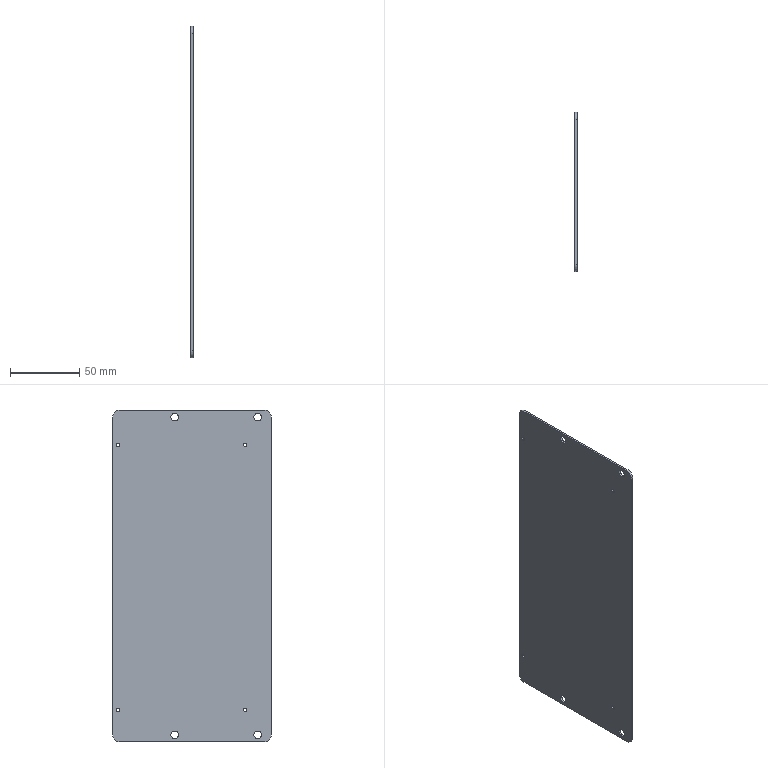Part | NX | features BREP 1 | 1 solid | 18 faces | box 1.5 x 115 x 240 mm | volume 41196 mm3 | cylinder 12 | plane 6 | commonest cylinder face diameters 2.5 x4 5.5 x4 10 x4
STEP:
#1=CARTESIAN_POINT('',(0.,-47.5,117.75));
#2=VERTEX_POINT('',#1);
#3=CARTESIAN_POINT('',(0.,-47.5,115.));
#4=DIRECTION('',(-1.,0.,0.));
#5=DIRECTION('',(0.,0.,1.));
#6=AXIS2_PLACEMENT_3D('',#3,#4,#5);
#7=CIRCLE('',#6,2.75);
#8=EDGE_CURVE('',#2,#2,#7,.T.);
#9=ORIENTED_EDGE('',*,*,#8,.T.);
#10=EDGE_LOOP('',(#9));
#11=FACE_BOUND('',#10,.T.);
#12=CARTESIAN_POINT('',(1.5,-47.5,117.75));
#13=VERTEX_POINT('',#12);
#14=CARTESIAN_POINT('',(1.5,-47.5,115.));
#15=DIRECTION('',(-1.,0.,0.));
#16=DIRECTION('',(0.,0.,1.));
#17=AXIS2_PLACEMENT_3D('',#14,#15,#16);
#18=CIRCLE('',#17,2.75);
#19=EDGE_CURVE('',#13,#13,#18,.T.);
#20=ORIENTED_EDGE('',*,*,#19,.F.);
#21=EDGE_LOOP('',(#20));
#22=FACE_BOUND('',#21,.T.);
#23=CARTESIAN_POINT('',(0.,-47.5,115.));
#24=DIRECTION('',(-1.,0.,0.));
#25=DIRECTION('',(0.,0.,1.));
#26=AXIS2_PLACEMENT_3D('',#23,#24,#25);
#27=CYLINDRICAL_SURFACE('',#26,2.75);
#28=ADVANCED_FACE('',(#11,#22),#27,.F.);
#29=CARTESIAN_POINT('',(0.,12.5,-112.25));
#30=VERTEX_POINT('',#29);
#31=CARTESIAN_POINT('',(0.,12.5,-115.));
#32=DIRECTION('',(-1.,0.,0.));
#33=DIRECTION('',(0.,0.,1.));
#34=AXIS2_PLACEMENT_3D('',#31,#32,#33);
#35=CIRCLE('',#34,2.75);
#36=EDGE_CURVE('',#30,#30,#35,.T.);
#37=ORIENTED_EDGE('',*,*,#36,.T.);
#38=EDGE_LOOP('',(#37));
#39=FACE_BOUND('',#38,.T.);
#40=CARTESIAN_POINT('',(1.5,12.5,-112.25));
#41=VERTEX_POINT('',#40);
#42=CARTESIAN_POINT('',(1.5,12.5,-115.));
#43=DIRECTION('',(-1.,0.,0.));
#44=DIRECTION('',(0.,0.,1.));
#45=AXIS2_PLACEMENT_3D('',#42,#43,#44);
#46=CIRCLE('',#45,2.75);
#47=EDGE_CURVE('',#41,#41,#46,.T.);
#48=ORIENTED_EDGE('',*,*,#47,.F.);
#49=EDGE_LOOP('',(#48));
#50=FACE_BOUND('',#49,.T.);
#51=CARTESIAN_POINT('',(0.,12.5,-115.));
#52=DIRECTION('',(-1.,0.,0.));
#53=DIRECTION('',(0.,0.,1.));
#54=AXIS2_PLACEMENT_3D('',#51,#52,#53);
#55=CYLINDRICAL_SURFACE('',#54,2.75);
#56=ADVANCED_FACE('',(#39,#50),#55,.F.);
#57=CARTESIAN_POINT('',(0.,-47.5,-112.25));
#58=VERTEX_POINT('',#57);
#59=CARTESIAN_POINT('',(0.,-47.5,-115.));
#60=DIRECTION('',(-1.,0.,0.));
#61=DIRECTION('',(0.,0.,1.));
#62=AXIS2_PLACEMENT_3D('',#59,#60,#61);
#63=CIRCLE('',#62,2.75);
#64=EDGE_CURVE('',#58,#58,#63,.T.);
#65=ORIENTED_EDGE('',*,*,#64,.T.);
#66=EDGE_LOOP('',(#65));
#67=FACE_BOUND('',#66,.T.);
#68=CARTESIAN_POINT('',(1.5,-47.5,-112.25));
#69=VERTEX_POINT('',#68);
#70=CARTESIAN_POINT('',(1.5,-47.5,-115.));
#71=DIRECTION('',(-1.,0.,0.));
#72=DIRECTION('',(0.,0.,1.));
#73=AXIS2_PLACEMENT_3D('',#70,#71,#72);
#74=CIRCLE('',#73,2.75);
#75=EDGE_CURVE('',#69,#69,#74,.T.);
#76=ORIENTED_EDGE('',*,*,#75,.F.);
#77=EDGE_LOOP('',(#76));
#78=FACE_BOUND('',#77,.T.);
#79=CARTESIAN_POINT('',(0.,-47.5,-115.));
#80=DIRECTION('',(-1.,0.,0.));
#81=DIRECTION('',(0.,0.,1.));
#82=AXIS2_PLACEMENT_3D('',#79,#80,#81);
#83=CYLINDRICAL_SURFACE('',#82,2.75);
#84=ADVANCED_FACE('',(#67,#78),#83,.F.);
#85=CARTESIAN_POINT('',(0.,12.5,117.75));
#86=VERTEX_POINT('',#85);
#87=CARTESIAN_POINT('',(0.,12.5,115.));
#88=DIRECTION('',(-1.,0.,0.));
#89=DIRECTION('',(0.,0.,1.));
#90=AXIS2_PLACEMENT_3D('',#87,#88,#89);
#91=CIRCLE('',#90,2.75);
#92=EDGE_CURVE('',#86,#86,#91,.T.);
#93=ORIENTED_EDGE('',*,*,#92,.T.);
#94=EDGE_LOOP('',(#93));
#95=FACE_BOUND('',#94,.T.);
#96=CARTESIAN_POINT('',(1.5,12.5,117.75));
#97=VERTEX_POINT('',#96);
#98=CARTESIAN_POINT('',(1.5,12.5,115.));
#99=DIRECTION('',(-1.,0.,0.));
#100=DIRECTION('',(0.,0.,1.));
#101=AXIS2_PLACEMENT_3D('',#98,#99,#100);
#102=CIRCLE('',#101,2.75);
#103=EDGE_CURVE('',#97,#97,#102,.T.);
#104=ORIENTED_EDGE('',*,*,#103,.F.);
#105=EDGE_LOOP('',(#104));
#106=FACE_BOUND('',#105,.T.);
#107=CARTESIAN_POINT('',(0.,12.5,115.));
#108=DIRECTION('',(-1.,0.,0.));
#109=DIRECTION('',(0.,0.,1.));
#110=AXIS2_PLACEMENT_3D('',#107,#108,#109);
#111=CYLINDRICAL_SURFACE('',#110,2.75);
#112=ADVANCED_FACE('',(#95,#106),#111,.F.);
#113=CARTESIAN_POINT('',(0.,53.5,96.25));
#114=VERTEX_POINT('',#113);
#115=CARTESIAN_POINT('',(0.,53.5,95.));
#116=DIRECTION('',(-1.,0.,0.));
#117=DIRECTION('',(0.,0.,1.));
#118=AXIS2_PLACEMENT_3D('',#115,#116,#117);
#119=CIRCLE('',#118,1.25);
#120=EDGE_CURVE('',#114,#114,#119,.T.);
#121=ORIENTED_EDGE('',*,*,#120,.T.);
#122=EDGE_LOOP('',(#121));
#123=FACE_BOUND('',#122,.T.);
#124=CARTESIAN_POINT('',(1.5,53.5,96.25));
#125=VERTEX_POINT('',#124);
#126=CARTESIAN_POINT('',(1.5,53.5,95.));
#127=DIRECTION('',(-1.,0.,0.));
#128=DIRECTION('',(0.,0.,1.));
#129=AXIS2_PLACEMENT_3D('',#126,#127,#128);
#130=CIRCLE('',#129,1.25);
#131=EDGE_CURVE('',#125,#125,#130,.T.);
#132=ORIENTED_EDGE('',*,*,#131,.F.);
#133=EDGE_LOOP('',(#132));
#134=FACE_BOUND('',#133,.T.);
#135=CARTESIAN_POINT('',(0.,53.5,95.));
#136=DIRECTION('',(-1.,0.,0.));
#137=DIRECTION('',(0.,0.,1.));
#138=AXIS2_PLACEMENT_3D('',#135,#136,#137);
#139=CYLINDRICAL_SURFACE('',#138,1.25);
#140=ADVANCED_FACE('',(#123,#134),#139,.F.);
#141=CARTESIAN_POINT('',(0.,53.5,-95.75));
#142=VERTEX_POINT('',#141);
#143=CARTESIAN_POINT('',(0.,53.5,-97.));
#144=DIRECTION('',(-1.,0.,0.));
#145=DIRECTION('',(0.,0.,1.));
#146=AXIS2_PLACEMENT_3D('',#143,#144,#145);
#147=CIRCLE('',#146,1.25);
#148=EDGE_CURVE('',#142,#142,#147,.T.);
#149=ORIENTED_EDGE('',*,*,#148,.T.);
#150=EDGE_LOOP('',(#149));
#151=FACE_BOUND('',#150,.T.);
#152=CARTESIAN_POINT('',(1.5,53.5,-95.75));
#153=VERTEX_POINT('',#152);
#154=CARTESIAN_POINT('',(1.5,53.5,-97.));
#155=DIRECTION('',(-1.,0.,0.));
#156=DIRECTION('',(0.,0.,1.));
#157=AXIS2_PLACEMENT_3D('',#154,#155,#156);
#158=CIRCLE('',#157,1.25);
#159=EDGE_CURVE('',#153,#153,#158,.T.);
#160=ORIENTED_EDGE('',*,*,#159,.F.);
#161=EDGE_LOOP('',(#160));
#162=FACE_BOUND('',#161,.T.);
#163=CARTESIAN_POINT('',(0.,53.5,-97.));
#164=DIRECTION('',(-1.,0.,0.));
#165=DIRECTION('',(0.,0.,1.));
#166=AXIS2_PLACEMENT_3D('',#163,#164,#165);
#167=CYLINDRICAL_SURFACE('',#166,1.25);
#168=ADVANCED_FACE('',(#151,#162),#167,.F.);
#169=CARTESIAN_POINT('',(0.,-38.5,-95.75));
#170=VERTEX_POINT('',#169);
#171=CARTESIAN_POINT('',(0.,-38.5,-97.));
#172=DIRECTION('',(-1.,0.,0.));
#173=DIRECTION('',(0.,0.,1.));
#174=AXIS2_PLACEMENT_3D('',#171,#172,#173);
#175=CIRCLE('',#174,1.25);
#176=EDGE_CURVE('',#170,#170,#175,.T.);
#177=ORIENTED_EDGE('',*,*,#176,.T.);
#178=EDGE_LOOP('',(#177));
#179=FACE_BOUND('',#178,.T.);
#180=CARTESIAN_POINT('',(1.5,-38.5,-95.75));
#181=VERTEX_POINT('',#180);
#182=CARTESIAN_POINT('',(1.5,-38.5,-97.));
#183=DIRECTION('',(-1.,0.,0.));
#184=DIRECTION('',(0.,0.,1.));
#185=AXIS2_PLACEMENT_3D('',#182,#183,#184);
#186=CIRCLE('',#185,1.25);
#187=EDGE_CURVE('',#181,#181,#186,.T.);
#188=ORIENTED_EDGE('',*,*,#187,.F.);
#189=EDGE_LOOP('',(#188));
#190=FACE_BOUND('',#189,.T.);
#191=CARTESIAN_POINT('',(0.,-38.5,-97.));
#192=DIRECTION('',(-1.,0.,0.));
#193=DIRECTION('',(0.,0.,1.));
#194=AXIS2_PLACEMENT_3D('',#191,#192,#193);
#195=CYLINDRICAL_SURFACE('',#194,1.25);
#196=ADVANCED_FACE('',(#179,#190),#195,.F.);
#197=CARTESIAN_POINT('',(0.,-38.5,96.25));
#198=VERTEX_POINT('',#197);
#199=CARTESIAN_POINT('',(0.,-38.5,95.));
#200=DIRECTION('',(-1.,0.,0.));
#201=DIRECTION('',(0.,0.,1.));
#202=AXIS2_PLACEMENT_3D('',#199,#200,#201);
#203=CIRCLE('',#202,1.25);
#204=EDGE_CURVE('',#198,#198,#203,.T.);
#205=ORIENTED_EDGE('',*,*,#204,.T.);
#206=EDGE_LOOP('',(#205));
#207=FACE_BOUND('',#206,.T.);
#208=CARTESIAN_POINT('',(1.5,-38.5,96.25));
#209=VERTEX_POINT('',#208);
#210=CARTESIAN_POINT('',(1.5,-38.5,95.));
#211=DIRECTION('',(-1.,0.,0.));
#212=DIRECTION('',(0.,0.,1.));
#213=AXIS2_PLACEMENT_3D('',#210,#211,#212);
#214=CIRCLE('',#213,1.25);
#215=EDGE_CURVE('',#209,#209,#214,.T.);
#216=ORIENTED_EDGE('',*,*,#215,.F.);
#217=EDGE_LOOP('',(#216));
#218=FACE_BOUND('',#217,.T.);
#219=CARTESIAN_POINT('',(0.,-38.5,95.));
#220=DIRECTION('',(-1.,0.,0.));
#221=DIRECTION('',(0.,0.,1.));
#222=AXIS2_PLACEMENT_3D('',#219,#220,#221);
#223=CYLINDRICAL_SURFACE('',#222,1.25);
#224=ADVANCED_FACE('',(#207,#218),#223,.F.);
#225=ORIENTED_EDGE('',*,*,#19,.T.);
#226=EDGE_LOOP('',(#225));
#227=FACE_BOUND('',#226,.T.);
#228=ORIENTED_EDGE('',*,*,#47,.T.);
#229=EDGE_LOOP('',(#228));
#230=FACE_BOUND('',#229,.T.);
#231=ORIENTED_EDGE('',*,*,#75,.T.);
#232=EDGE_LOOP('',(#231));
#233=FACE_BOUND('',#232,.T.);
#234=ORIENTED_EDGE('',*,*,#103,.T.);
#235=EDGE_LOOP('',(#234));
#236=FACE_BOUND('',#235,.T.);
#237=CARTESIAN_POINT('',(1.5,-52.5,-120.));
#238=VERTEX_POINT('',#237);
#239=CARTESIAN_POINT('',(1.5,52.5,-120.));
#240=VERTEX_POINT('',#239);
#241=CARTESIAN_POINT('',(1.5,57.5,-120.));
#242=DIRECTION('',(0.,1.,0.));
#243=VECTOR('',#242,1000.);
#244=LINE('',#241,#243);
#245=EDGE_CURVE('',#238,#240,#244,.T.);
#246=ORIENTED_EDGE('',*,*,#245,.T.);
#247=CARTESIAN_POINT('',(1.5,57.5,-115.));
#248=VERTEX_POINT('',#247);
#249=CARTESIAN_POINT('',(1.5,52.5,-115.));
#250=DIRECTION('',(1.,0.,0.));
#251=DIRECTION('',(0.,0.,-1.));
#252=AXIS2_PLACEMENT_3D('',#249,#250,#251);
#253=CIRCLE('',#252,5.);
#254=EDGE_CURVE('',#240,#248,#253,.T.);
#255=ORIENTED_EDGE('',*,*,#254,.T.);
#256=CARTESIAN_POINT('',(1.5,57.5,115.));
#257=VERTEX_POINT('',#256);
#258=CARTESIAN_POINT('',(1.5,57.5,120.));
#259=DIRECTION('',(0.,0.,1.));
#260=VECTOR('',#259,1000.);
#261=LINE('',#258,#260);
#262=EDGE_CURVE('',#248,#257,#261,.T.);
#263=ORIENTED_EDGE('',*,*,#262,.T.);
#264=CARTESIAN_POINT('',(1.5,52.5,120.));
#265=VERTEX_POINT('',#264);
#266=CARTESIAN_POINT('',(1.5,52.5,115.));
#267=DIRECTION('',(1.,0.,0.));
#268=DIRECTION('',(0.,0.,-1.));
#269=AXIS2_PLACEMENT_3D('',#266,#267,#268);
#270=CIRCLE('',#269,5.);
#271=EDGE_CURVE('',#257,#265,#270,.T.);
#272=ORIENTED_EDGE('',*,*,#271,.T.);
#273=CARTESIAN_POINT('',(1.5,-52.5,120.));
#274=VERTEX_POINT('',#273);
#275=CARTESIAN_POINT('',(1.5,57.5,120.));
#276=DIRECTION('',(0.,-1.,0.));
#277=VECTOR('',#276,1000.);
#278=LINE('',#275,#277);
#279=EDGE_CURVE('',#265,#274,#278,.T.);
#280=ORIENTED_EDGE('',*,*,#279,.T.);
#281=CARTESIAN_POINT('',(1.5,-57.5,115.));
#282=VERTEX_POINT('',#281);
#283=CARTESIAN_POINT('',(1.5,-52.5,115.));
#284=DIRECTION('',(1.,0.,0.));
#285=DIRECTION('',(0.,0.,-1.));
#286=AXIS2_PLACEMENT_3D('',#283,#284,#285);
#287=CIRCLE('',#286,5.);
#288=EDGE_CURVE('',#274,#282,#287,.T.);
#289=ORIENTED_EDGE('',*,*,#288,.T.);
#290=CARTESIAN_POINT('',(1.5,-57.5,-115.));
#291=VERTEX_POINT('',#290);
#292=CARTESIAN_POINT('',(1.5,-57.5,120.));
#293=DIRECTION('',(0.,0.,-1.));
#294=VECTOR('',#293,1000.);
#295=LINE('',#292,#294);
#296=EDGE_CURVE('',#282,#291,#295,.T.);
#297=ORIENTED_EDGE('',*,*,#296,.T.);
#298=CARTESIAN_POINT('',(1.5,-52.5,-115.));
#299=DIRECTION('',(1.,0.,0.));
#300=DIRECTION('',(0.,0.,-1.));
#301=AXIS2_PLACEMENT_3D('',#298,#299,#300);
#302=CIRCLE('',#301,5.);
#303=EDGE_CURVE('',#291,#238,#302,.T.);
#304=ORIENTED_EDGE('',*,*,#303,.T.);
#305=EDGE_LOOP('',(#246,#255,#263,#272,#280,#289,#297,#304));
#306=FACE_BOUND('',#305,.T.);
#307=ORIENTED_EDGE('',*,*,#215,.T.);
#308=EDGE_LOOP('',(#307));
#309=FACE_BOUND('',#308,.T.);
#310=ORIENTED_EDGE('',*,*,#187,.T.);
#311=EDGE_LOOP('',(#310));
#312=FACE_BOUND('',#311,.T.);
#313=ORIENTED_EDGE('',*,*,#159,.T.);
#314=EDGE_LOOP('',(#313));
#315=FACE_BOUND('',#314,.T.);
#316=ORIENTED_EDGE('',*,*,#131,.T.);
#317=EDGE_LOOP('',(#316));
#318=FACE_BOUND('',#317,.T.);
#319=CARTESIAN_POINT('',(1.5,0.,0.));
#320=DIRECTION('',(1.,0.,0.));
#321=DIRECTION('',(0.,0.,-1.));
#322=AXIS2_PLACEMENT_3D('',#319,#320,#321);
#323=PLANE('',#322);
#324=ADVANCED_FACE('',(#227,#230,#233,#236,#306,#309,#312,#315,#318),#323,.T.);
#325=CARTESIAN_POINT('',(0.,-52.5,-120.));
#326=VERTEX_POINT('',#325);
#327=CARTESIAN_POINT('',(0.,52.5,-120.));
#328=VERTEX_POINT('',#327);
#329=CARTESIAN_POINT('',(0.,57.5,-120.));
#330=DIRECTION('',(0.,1.,0.));
#331=VECTOR('',#330,1000.);
#332=LINE('',#329,#331);
#333=EDGE_CURVE('',#326,#328,#332,.T.);
#334=ORIENTED_EDGE('',*,*,#333,.T.);
#335=CARTESIAN_POINT('',(1.5,52.5,-120.));
#336=DIRECTION('',(1.,0.,0.));
#337=VECTOR('',#336,1000.);
#338=LINE('',#335,#337);
#339=EDGE_CURVE('',#328,#240,#338,.T.);
#340=ORIENTED_EDGE('',*,*,#339,.T.);
#341=ORIENTED_EDGE('',*,*,#245,.F.);
#342=CARTESIAN_POINT('',(1.5,-52.5,-120.));
#343=DIRECTION('',(-1.,0.,0.));
#344=VECTOR('',#343,1000.);
#345=LINE('',#342,#344);
#346=EDGE_CURVE('',#238,#326,#345,.T.);
#347=ORIENTED_EDGE('',*,*,#346,.T.);
#348=EDGE_LOOP('',(#334,#340,#341,#347));
#349=FACE_BOUND('',#348,.T.);
#350=CARTESIAN_POINT('',(1.5,57.5,-120.));
#351=DIRECTION('',(0.,0.,1.));
#352=DIRECTION('',(1.,0.,0.));
#353=AXIS2_PLACEMENT_3D('',#350,#351,#352);
#354=PLANE('',#353);
#355=ADVANCED_FACE('',(#349),#354,.F.);
#356=ORIENTED_EDGE('',*,*,#262,.F.);
#357=CARTESIAN_POINT('',(0.,57.5,-115.));
#358=VERTEX_POINT('',#357);
#359=CARTESIAN_POINT('',(1.5,57.5,-115.));
#360=DIRECTION('',(-1.,0.,0.));
#361=VECTOR('',#360,1000.);
#362=LINE('',#359,#361);
#363=EDGE_CURVE('',#248,#358,#362,.T.);
#364=ORIENTED_EDGE('',*,*,#363,.T.);
#365=CARTESIAN_POINT('',(0.,57.5,115.));
#366=VERTEX_POINT('',#365);
#367=CARTESIAN_POINT('',(0.,57.5,120.));
#368=DIRECTION('',(0.,0.,1.));
#369=VECTOR('',#368,1000.);
#370=LINE('',#367,#369);
#371=EDGE_CURVE('',#358,#366,#370,.T.);
#372=ORIENTED_EDGE('',*,*,#371,.T.);
#373=CARTESIAN_POINT('',(1.5,57.5,115.));
#374=DIRECTION('',(1.,0.,0.));
#375=VECTOR('',#374,1000.);
#376=LINE('',#373,#375);
#377=EDGE_CURVE('',#366,#257,#376,.T.);
#378=ORIENTED_EDGE('',*,*,#377,.T.);
#379=EDGE_LOOP('',(#356,#364,#372,#378));
#380=FACE_BOUND('',#379,.T.);
#381=CARTESIAN_POINT('',(1.5,57.5,120.));
#382=DIRECTION('',(0.,-1.,0.));
#383=DIRECTION('',(0.,0.,-1.));
#384=AXIS2_PLACEMENT_3D('',#381,#382,#383);
#385=PLANE('',#384);
#386=ADVANCED_FACE('',(#380),#385,.F.);
#387=CARTESIAN_POINT('',(0.,52.5,120.));
#388=VERTEX_POINT('',#387);
#389=CARTESIAN_POINT('',(0.,-52.5,120.));
#390=VERTEX_POINT('',#389);
#391=CARTESIAN_POINT('',(0.,57.5,120.));
#392=DIRECTION('',(0.,-1.,0.));
#393=VECTOR('',#392,1000.);
#394=LINE('',#391,#393);
#395=EDGE_CURVE('',#388,#390,#394,.T.);
#396=ORIENTED_EDGE('',*,*,#395,.T.);
#397=CARTESIAN_POINT('',(1.5,-52.5,120.));
#398=DIRECTION('',(1.,0.,0.));
#399=VECTOR('',#398,1000.);
#400=LINE('',#397,#399);
#401=EDGE_CURVE('',#390,#274,#400,.T.);
#402=ORIENTED_EDGE('',*,*,#401,.T.);
#403=ORIENTED_EDGE('',*,*,#279,.F.);
#404=CARTESIAN_POINT('',(1.5,52.5,120.));
#405=DIRECTION('',(-1.,0.,0.));
#406=VECTOR('',#405,1000.);
#407=LINE('',#404,#406);
#408=EDGE_CURVE('',#265,#388,#407,.T.);
#409=ORIENTED_EDGE('',*,*,#408,.T.);
#410=EDGE_LOOP('',(#396,#402,#403,#409));
#411=FACE_BOUND('',#410,.T.);
#412=CARTESIAN_POINT('',(1.5,57.5,120.));
#413=DIRECTION('',(0.,0.,-1.));
#414=DIRECTION('',(-1.,0.,0.));
#415=AXIS2_PLACEMENT_3D('',#412,#413,#414);
#416=PLANE('',#415);
#417=ADVANCED_FACE('',(#411),#416,.F.);
#418=CARTESIAN_POINT('',(0.,-57.5,115.));
#419=VERTEX_POINT('',#418);
#420=CARTESIAN_POINT('',(0.,-57.5,-115.));
#421=VERTEX_POINT('',#420);
#422=CARTESIAN_POINT('',(0.,-57.5,120.));
#423=DIRECTION('',(0.,0.,-1.));
#424=VECTOR('',#423,1000.);
#425=LINE('',#422,#424);
#426=EDGE_CURVE('',#419,#421,#425,.T.);
#427=ORIENTED_EDGE('',*,*,#426,.T.);
#428=CARTESIAN_POINT('',(1.5,-57.5,-115.));
#429=DIRECTION('',(1.,0.,0.));
#430=VECTOR('',#429,1000.);
#431=LINE('',#428,#430);
#432=EDGE_CURVE('',#421,#291,#431,.T.);
#433=ORIENTED_EDGE('',*,*,#432,.T.);
#434=ORIENTED_EDGE('',*,*,#296,.F.);
#435=CARTESIAN_POINT('',(1.5,-57.5,115.));
#436=DIRECTION('',(-1.,0.,0.));
#437=VECTOR('',#436,1000.);
#438=LINE('',#435,#437);
#439=EDGE_CURVE('',#282,#419,#438,.T.);
#440=ORIENTED_EDGE('',*,*,#439,.T.);
#441=EDGE_LOOP('',(#427,#433,#434,#440));
#442=FACE_BOUND('',#441,.T.);
#443=CARTESIAN_POINT('',(1.5,-57.5,120.));
#444=DIRECTION('',(0.,1.,0.));
#445=DIRECTION('',(0.,0.,1.));
#446=AXIS2_PLACEMENT_3D('',#443,#444,#445);
#447=PLANE('',#446);
#448=ADVANCED_FACE('',(#442),#447,.F.);
#449=ORIENTED_EDGE('',*,*,#8,.F.);
#450=EDGE_LOOP('',(#449));
#451=FACE_BOUND('',#450,.T.);
#452=ORIENTED_EDGE('',*,*,#36,.F.);
#453=EDGE_LOOP('',(#452));
#454=FACE_BOUND('',#453,.T.);
#455=ORIENTED_EDGE('',*,*,#64,.F.);
#456=EDGE_LOOP('',(#455));
#457=FACE_BOUND('',#456,.T.);
#458=ORIENTED_EDGE('',*,*,#92,.F.);
#459=EDGE_LOOP('',(#458));
#460=FACE_BOUND('',#459,.T.);
#461=ORIENTED_EDGE('',*,*,#120,.F.);
#462=EDGE_LOOP('',(#461));
#463=FACE_BOUND('',#462,.T.);
#464=ORIENTED_EDGE('',*,*,#148,.F.);
#465=EDGE_LOOP('',(#464));
#466=FACE_BOUND('',#465,.T.);
#467=ORIENTED_EDGE('',*,*,#176,.F.);
#468=EDGE_LOOP('',(#467));
#469=FACE_BOUND('',#468,.T.);
#470=ORIENTED_EDGE('',*,*,#204,.F.);
#471=EDGE_LOOP('',(#470));
#472=FACE_BOUND('',#471,.T.);
#473=ORIENTED_EDGE('',*,*,#371,.F.);
#474=CARTESIAN_POINT('',(0.,52.5,-115.));
#475=DIRECTION('',(-1.,0.,0.));
#476=DIRECTION('',(0.,0.,-1.));
#477=AXIS2_PLACEMENT_3D('',#474,#475,#476);
#478=CIRCLE('',#477,5.);
#479=EDGE_CURVE('',#358,#328,#478,.T.);
#480=ORIENTED_EDGE('',*,*,#479,.T.);
#481=ORIENTED_EDGE('',*,*,#333,.F.);
#482=CARTESIAN_POINT('',(0.,-52.5,-115.));
#483=DIRECTION('',(-1.,0.,0.));
#484=DIRECTION('',(0.,0.,-1.));
#485=AXIS2_PLACEMENT_3D('',#482,#483,#484);
#486=CIRCLE('',#485,5.);
#487=EDGE_CURVE('',#326,#421,#486,.T.);
#488=ORIENTED_EDGE('',*,*,#487,.T.);
#489=ORIENTED_EDGE('',*,*,#426,.F.);
#490=CARTESIAN_POINT('',(0.,-52.5,115.));
#491=DIRECTION('',(-1.,0.,0.));
#492=DIRECTION('',(0.,0.,-1.));
#493=AXIS2_PLACEMENT_3D('',#490,#491,#492);
#494=CIRCLE('',#493,5.);
#495=EDGE_CURVE('',#419,#390,#494,.T.);
#496=ORIENTED_EDGE('',*,*,#495,.T.);
#497=ORIENTED_EDGE('',*,*,#395,.F.);
#498=CARTESIAN_POINT('',(0.,52.5,115.));
#499=DIRECTION('',(-1.,0.,0.));
#500=DIRECTION('',(0.,0.,-1.));
#501=AXIS2_PLACEMENT_3D('',#498,#499,#500);
#502=CIRCLE('',#501,5.);
#503=EDGE_CURVE('',#388,#366,#502,.T.);
#504=ORIENTED_EDGE('',*,*,#503,.T.);
#505=EDGE_LOOP('',(#473,#480,#481,#488,#489,#496,#497,#504));
#506=FACE_BOUND('',#505,.T.);
#507=CARTESIAN_POINT('',(0.,0.,0.));
#508=DIRECTION('',(1.,0.,0.));
#509=DIRECTION('',(0.,0.,-1.));
#510=AXIS2_PLACEMENT_3D('',#507,#508,#509);
#511=PLANE('',#510);
#512=ADVANCED_FACE('',(#451,#454,#457,#460,#463,#466,#469,#472,#506),#511,.F.);
#513=ORIENTED_EDGE('',*,*,#254,.F.);
#514=ORIENTED_EDGE('',*,*,#339,.F.);
#515=ORIENTED_EDGE('',*,*,#479,.F.);
#516=ORIENTED_EDGE('',*,*,#363,.F.);
#517=EDGE_LOOP('',(#513,#514,#515,#516));
#518=FACE_BOUND('',#517,.T.);
#519=CARTESIAN_POINT('',(1.5,52.5,-115.));
#520=DIRECTION('',(-1.,0.,0.));
#521=DIRECTION('',(0.,0.,1.));
#522=AXIS2_PLACEMENT_3D('',#519,#520,#521);
#523=CYLINDRICAL_SURFACE('',#522,5.);
#524=ADVANCED_FACE('',(#518),#523,.T.);
#525=ORIENTED_EDGE('',*,*,#303,.F.);
#526=ORIENTED_EDGE('',*,*,#432,.F.);
#527=ORIENTED_EDGE('',*,*,#487,.F.);
#528=ORIENTED_EDGE('',*,*,#346,.F.);
#529=EDGE_LOOP('',(#525,#526,#527,#528));
#530=FACE_BOUND('',#529,.T.);
#531=CARTESIAN_POINT('',(1.5,-52.5,-115.));
#532=DIRECTION('',(-1.,0.,0.));
#533=DIRECTION('',(0.,0.,1.));
#534=AXIS2_PLACEMENT_3D('',#531,#532,#533);
#535=CYLINDRICAL_SURFACE('',#534,5.);
#536=ADVANCED_FACE('',(#530),#535,.T.);
#537=ORIENTED_EDGE('',*,*,#288,.F.);
#538=ORIENTED_EDGE('',*,*,#401,.F.);
#539=ORIENTED_EDGE('',*,*,#495,.F.);
#540=ORIENTED_EDGE('',*,*,#439,.F.);
#541=EDGE_LOOP('',(#537,#538,#539,#540));
#542=FACE_BOUND('',#541,.T.);
#543=CARTESIAN_POINT('',(1.5,-52.5,115.));
#544=DIRECTION('',(-1.,0.,0.));
#545=DIRECTION('',(0.,0.,1.));
#546=AXIS2_PLACEMENT_3D('',#543,#544,#545);
#547=CYLINDRICAL_SURFACE('',#546,5.);
#548=ADVANCED_FACE('',(#542),#547,.T.);
#549=ORIENTED_EDGE('',*,*,#271,.F.);
#550=ORIENTED_EDGE('',*,*,#377,.F.);
#551=ORIENTED_EDGE('',*,*,#503,.F.);
#552=ORIENTED_EDGE('',*,*,#408,.F.);
#553=EDGE_LOOP('',(#549,#550,#551,#552));
#554=FACE_BOUND('',#553,.T.);
#555=CARTESIAN_POINT('',(1.5,52.5,115.));
#556=DIRECTION('',(-1.,0.,0.));
#557=DIRECTION('',(0.,0.,1.));
#558=AXIS2_PLACEMENT_3D('',#555,#556,#557);
#559=CYLINDRICAL_SURFACE('',#558,5.);
#560=ADVANCED_FACE('',(#554),#559,.T.);
#561=CLOSED_SHELL('',(#28,#56,#84,#112,#140,#168,#196,#224,#324,#355,#386,#417,#448,#512,#524,#536,#548,#560));
#562=MANIFOLD_SOLID_BREP('',#561);
#563=(LENGTH_UNIT()NAMED_UNIT(*)SI_UNIT(.MILLI.,.METRE.));
#564=UNCERTAINTY_MEASURE_WITH_UNIT(LENGTH_MEASURE(0.00001),#563,'','');
#565=(NAMED_UNIT(*)PLANE_ANGLE_UNIT()SI_UNIT($,.RADIAN.));
#566=(NAMED_UNIT(*)SI_UNIT($,.STERADIAN.)SOLID_ANGLE_UNIT());
#567=(GEOMETRIC_REPRESENTATION_CONTEXT(3)GLOBAL_UNCERTAINTY_ASSIGNED_CONTEXT((#564))GLOBAL_UNIT_ASSIGNED_CONTEXT((#563,#565,#566))REPRESENTATION_CONTEXT('',''));
#568=ADVANCED_BREP_SHAPE_REPRESENTATION('',(#562),#567);